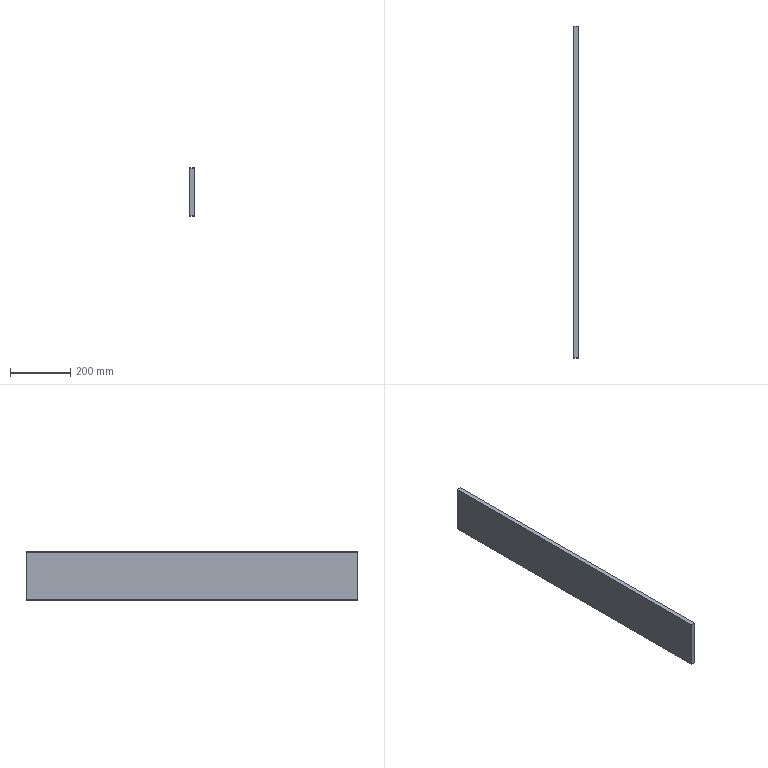Part | STEP file | HJDX-204 | 1 solid | 26 faces | box 16 x 1100 x 160 mm | volume 2815363 mm3 | plane 26
STEP:
#1=CARTESIAN_POINT('',(16.,-549.5,-79.5));
#2=VERTEX_POINT('',#1);
#3=CARTESIAN_POINT('',(16.,-549.5,79.5));
#4=VERTEX_POINT('',#3);
#5=CARTESIAN_POINT('',(16.,-549.5,0.));
#6=DIRECTION('',(0.,0.,1.));
#7=VECTOR('',#6,1000.);
#8=LINE('',#5,#7);
#9=EDGE_CURVE('',#2,#4,#8,.T.);
#10=ORIENTED_EDGE('',*,*,#9,.F.);
#11=CARTESIAN_POINT('',(16.,549.5,-79.5));
#12=VERTEX_POINT('',#11);
#13=CARTESIAN_POINT('',(16.,0.,-79.5));
#14=DIRECTION('',(0.,-1.,0.));
#15=VECTOR('',#14,1000.);
#16=LINE('',#13,#15);
#17=EDGE_CURVE('',#12,#2,#16,.T.);
#18=ORIENTED_EDGE('',*,*,#17,.F.);
#19=CARTESIAN_POINT('',(16.,549.5,79.5));
#20=VERTEX_POINT('',#19);
#21=CARTESIAN_POINT('',(16.,549.5,0.));
#22=DIRECTION('',(0.,0.,-1.));
#23=VECTOR('',#22,1000.);
#24=LINE('',#21,#23);
#25=EDGE_CURVE('',#20,#12,#24,.T.);
#26=ORIENTED_EDGE('',*,*,#25,.F.);
#27=CARTESIAN_POINT('',(16.,0.,79.5));
#28=DIRECTION('',(0.,1.,0.));
#29=VECTOR('',#28,1000.);
#30=LINE('',#27,#29);
#31=EDGE_CURVE('',#4,#20,#30,.T.);
#32=ORIENTED_EDGE('',*,*,#31,.F.);
#33=EDGE_LOOP('',(#10,#18,#26,#32));
#34=FACE_OUTER_BOUND('',#33,.T.);
#35=CARTESIAN_POINT('',(16.,0.,0.));
#36=DIRECTION('',(-1.,0.,0.));
#37=DIRECTION('',(0.,0.,1.));
#38=AXIS2_PLACEMENT_3D('',#35,#36,#37);
#39=PLANE('',#38);
#40=ADVANCED_FACE('',(#34),#39,.F.);
#41=CARTESIAN_POINT('',(15.5,-549.5,80.));
#42=VERTEX_POINT('',#41);
#43=CARTESIAN_POINT('',(15.5,549.5,80.));
#44=VERTEX_POINT('',#43);
#45=CARTESIAN_POINT('',(15.5,0.,80.));
#46=DIRECTION('',(0.,1.,0.));
#47=VECTOR('',#46,1000.);
#48=LINE('',#45,#47);
#49=EDGE_CURVE('',#42,#44,#48,.T.);
#50=ORIENTED_EDGE('',*,*,#49,.F.);
#51=CARTESIAN_POINT('',(16.,-549.5,79.5));
#52=DIRECTION('',(-0.7071,0.,0.7071));
#53=VECTOR('',#52,1000.);
#54=LINE('',#51,#53);
#55=EDGE_CURVE('',#4,#42,#54,.T.);
#56=ORIENTED_EDGE('',*,*,#55,.F.);
#57=ORIENTED_EDGE('',*,*,#31,.T.);
#58=CARTESIAN_POINT('',(16.,549.5,79.5));
#59=DIRECTION('',(0.7071,0.,-0.7071));
#60=VECTOR('',#59,1000.);
#61=LINE('',#58,#60);
#62=EDGE_CURVE('',#44,#20,#61,.T.);
#63=ORIENTED_EDGE('',*,*,#62,.F.);
#64=EDGE_LOOP('',(#50,#56,#57,#63));
#65=FACE_OUTER_BOUND('',#64,.T.);
#66=CARTESIAN_POINT('',(16.,0.,79.5));
#67=DIRECTION('',(-0.7071,0.,-0.7071));
#68=DIRECTION('',(-0.7071,0.,0.7071));
#69=AXIS2_PLACEMENT_3D('',#66,#67,#68);
#70=PLANE('',#69);
#71=ADVANCED_FACE('',(#65),#70,.F.);
#72=CARTESIAN_POINT('',(15.5,-550.,-79.5));
#73=VERTEX_POINT('',#72);
#74=CARTESIAN_POINT('',(15.5,-550.,79.5));
#75=VERTEX_POINT('',#74);
#76=CARTESIAN_POINT('',(15.5,-550.,0.));
#77=DIRECTION('',(0.,0.,1.));
#78=VECTOR('',#77,1000.);
#79=LINE('',#76,#78);
#80=EDGE_CURVE('',#73,#75,#79,.T.);
#81=ORIENTED_EDGE('',*,*,#80,.F.);
#82=CARTESIAN_POINT('',(16.,-549.5,-79.5));
#83=DIRECTION('',(-0.7071,-0.7071,0.));
#84=VECTOR('',#83,1000.);
#85=LINE('',#82,#84);
#86=EDGE_CURVE('',#2,#73,#85,.T.);
#87=ORIENTED_EDGE('',*,*,#86,.F.);
#88=ORIENTED_EDGE('',*,*,#9,.T.);
#89=CARTESIAN_POINT('',(16.,-549.5,79.5));
#90=DIRECTION('',(0.7071,0.7071,0.));
#91=VECTOR('',#90,1000.);
#92=LINE('',#89,#91);
#93=EDGE_CURVE('',#75,#4,#92,.T.);
#94=ORIENTED_EDGE('',*,*,#93,.F.);
#95=EDGE_LOOP('',(#81,#87,#88,#94));
#96=FACE_OUTER_BOUND('',#95,.T.);
#97=CARTESIAN_POINT('',(16.,-549.5,0.));
#98=DIRECTION('',(-0.7071,0.7071,0.));
#99=DIRECTION('',(-0.7071,-0.7071,0.));
#100=AXIS2_PLACEMENT_3D('',#97,#98,#99);
#101=PLANE('',#100);
#102=ADVANCED_FACE('',(#96),#101,.F.);
#103=ORIENTED_EDGE('',*,*,#17,.T.);
#104=CARTESIAN_POINT('',(15.5,-549.5,-80.));
#105=VERTEX_POINT('',#104);
#106=CARTESIAN_POINT('',(16.,-549.5,-79.5));
#107=DIRECTION('',(0.7071,0.,0.7071));
#108=VECTOR('',#107,1000.);
#109=LINE('',#106,#108);
#110=EDGE_CURVE('',#105,#2,#109,.T.);
#111=ORIENTED_EDGE('',*,*,#110,.F.);
#112=CARTESIAN_POINT('',(15.5,549.5,-80.));
#113=VERTEX_POINT('',#112);
#114=CARTESIAN_POINT('',(15.5,0.,-80.));
#115=DIRECTION('',(0.,-1.,0.));
#116=VECTOR('',#115,1000.);
#117=LINE('',#114,#116);
#118=EDGE_CURVE('',#113,#105,#117,.T.);
#119=ORIENTED_EDGE('',*,*,#118,.F.);
#120=CARTESIAN_POINT('',(16.,549.5,-79.5));
#121=DIRECTION('',(-0.7071,0.,-0.7071));
#122=VECTOR('',#121,1000.);
#123=LINE('',#120,#122);
#124=EDGE_CURVE('',#12,#113,#123,.T.);
#125=ORIENTED_EDGE('',*,*,#124,.F.);
#126=EDGE_LOOP('',(#103,#111,#119,#125));
#127=FACE_OUTER_BOUND('',#126,.T.);
#128=CARTESIAN_POINT('',(16.,0.,-79.5));
#129=DIRECTION('',(-0.7071,0.,0.7071));
#130=DIRECTION('',(0.7071,0.,0.7071));
#131=AXIS2_PLACEMENT_3D('',#128,#129,#130);
#132=PLANE('',#131);
#133=ADVANCED_FACE('',(#127),#132,.F.);
#134=ORIENTED_EDGE('',*,*,#25,.T.);
#135=CARTESIAN_POINT('',(15.5,550.,-79.5));
#136=VERTEX_POINT('',#135);
#137=CARTESIAN_POINT('',(16.,549.5,-79.5));
#138=DIRECTION('',(0.7071,-0.7071,0.));
#139=VECTOR('',#138,1000.);
#140=LINE('',#137,#139);
#141=EDGE_CURVE('',#136,#12,#140,.T.);
#142=ORIENTED_EDGE('',*,*,#141,.F.);
#143=CARTESIAN_POINT('',(15.5,550.,79.5));
#144=VERTEX_POINT('',#143);
#145=CARTESIAN_POINT('',(15.5,550.,0.));
#146=DIRECTION('',(0.,0.,-1.));
#147=VECTOR('',#146,1000.);
#148=LINE('',#145,#147);
#149=EDGE_CURVE('',#144,#136,#148,.T.);
#150=ORIENTED_EDGE('',*,*,#149,.F.);
#151=CARTESIAN_POINT('',(16.,549.5,79.5));
#152=DIRECTION('',(-0.7071,0.7071,0.));
#153=VECTOR('',#152,1000.);
#154=LINE('',#151,#153);
#155=EDGE_CURVE('',#20,#144,#154,.T.);
#156=ORIENTED_EDGE('',*,*,#155,.F.);
#157=EDGE_LOOP('',(#134,#142,#150,#156));
#158=FACE_OUTER_BOUND('',#157,.T.);
#159=CARTESIAN_POINT('',(16.,549.5,0.));
#160=DIRECTION('',(-0.7071,-0.7071,0.));
#161=DIRECTION('',(0.7071,-0.7071,0.));
#162=AXIS2_PLACEMENT_3D('',#159,#160,#161);
#163=PLANE('',#162);
#164=ADVANCED_FACE('',(#158),#163,.F.);
#165=CARTESIAN_POINT('',(15.5,549.5,80.));
#166=DIRECTION('',(0.,-0.7071,0.7071));
#167=VECTOR('',#166,1000.);
#168=LINE('',#165,#167);
#169=EDGE_CURVE('',#144,#44,#168,.T.);
#170=ORIENTED_EDGE('',*,*,#169,.T.);
#171=ORIENTED_EDGE('',*,*,#62,.T.);
#172=ORIENTED_EDGE('',*,*,#155,.T.);
#173=EDGE_LOOP('',(#170,#171,#172));
#174=FACE_OUTER_BOUND('',#173,.T.);
#175=CARTESIAN_POINT('',(15.5,550.,79.5));
#176=DIRECTION('',(0.5774,0.5774,0.5774));
#177=DIRECTION('',(0.7071,0.,-0.7071));
#178=AXIS2_PLACEMENT_3D('',#175,#176,#177);
#179=PLANE('',#178);
#180=ADVANCED_FACE('',(#174),#179,.T.);
#181=CARTESIAN_POINT('',(0.5,549.5,80.));
#182=VERTEX_POINT('',#181);
#183=CARTESIAN_POINT('',(16.,549.5,80.));
#184=DIRECTION('',(1.,0.,0.));
#185=VECTOR('',#184,1000.);
#186=LINE('',#183,#185);
#187=EDGE_CURVE('',#182,#44,#186,.T.);
#188=ORIENTED_EDGE('',*,*,#187,.F.);
#189=CARTESIAN_POINT('',(0.5,-549.5,80.));
#190=VERTEX_POINT('',#189);
#191=CARTESIAN_POINT('',(0.5,-550.,80.));
#192=DIRECTION('',(0.,1.,0.));
#193=VECTOR('',#192,1000.);
#194=LINE('',#191,#193);
#195=EDGE_CURVE('',#190,#182,#194,.T.);
#196=ORIENTED_EDGE('',*,*,#195,.F.);
#197=CARTESIAN_POINT('',(16.,-549.5,80.));
#198=DIRECTION('',(-1.,0.,0.));
#199=VECTOR('',#198,1000.);
#200=LINE('',#197,#199);
#201=EDGE_CURVE('',#42,#190,#200,.T.);
#202=ORIENTED_EDGE('',*,*,#201,.F.);
#203=ORIENTED_EDGE('',*,*,#49,.T.);
#204=EDGE_LOOP('',(#188,#196,#202,#203));
#205=FACE_OUTER_BOUND('',#204,.T.);
#206=CARTESIAN_POINT('',(16.,-550.,80.));
#207=DIRECTION('',(0.,0.,-1.));
#208=DIRECTION('',(-1.,0.,0.));
#209=AXIS2_PLACEMENT_3D('',#206,#207,#208);
#210=PLANE('',#209);
#211=ADVANCED_FACE('',(#205),#210,.F.);
#212=CARTESIAN_POINT('',(15.5,-549.5,80.));
#213=DIRECTION('',(0.,-0.7071,-0.7071));
#214=VECTOR('',#213,1000.);
#215=LINE('',#212,#214);
#216=EDGE_CURVE('',#42,#75,#215,.T.);
#217=ORIENTED_EDGE('',*,*,#216,.T.);
#218=ORIENTED_EDGE('',*,*,#93,.T.);
#219=ORIENTED_EDGE('',*,*,#55,.T.);
#220=EDGE_LOOP('',(#217,#218,#219));
#221=FACE_OUTER_BOUND('',#220,.T.);
#222=CARTESIAN_POINT('',(15.5,-549.5,80.));
#223=DIRECTION('',(0.5774,-0.5774,0.5774));
#224=DIRECTION('',(0.7071,0.,-0.7071));
#225=AXIS2_PLACEMENT_3D('',#222,#223,#224);
#226=PLANE('',#225);
#227=ADVANCED_FACE('',(#221),#226,.T.);
#228=CARTESIAN_POINT('',(0.5,-550.,-79.5));
#229=VERTEX_POINT('',#228);
#230=CARTESIAN_POINT('',(16.,-550.,-79.5));
#231=DIRECTION('',(-1.,0.,0.));
#232=VECTOR('',#231,1000.);
#233=LINE('',#230,#232);
#234=EDGE_CURVE('',#73,#229,#233,.T.);
#235=ORIENTED_EDGE('',*,*,#234,.F.);
#236=ORIENTED_EDGE('',*,*,#80,.T.);
#237=CARTESIAN_POINT('',(0.5,-550.,79.5));
#238=VERTEX_POINT('',#237);
#239=CARTESIAN_POINT('',(16.,-550.,79.5));
#240=DIRECTION('',(1.,0.,0.));
#241=VECTOR('',#240,1000.);
#242=LINE('',#239,#241);
#243=EDGE_CURVE('',#238,#75,#242,.T.);
#244=ORIENTED_EDGE('',*,*,#243,.F.);
#245=CARTESIAN_POINT('',(0.5,-550.,80.));
#246=DIRECTION('',(0.,0.,1.));
#247=VECTOR('',#246,1000.);
#248=LINE('',#245,#247);
#249=EDGE_CURVE('',#229,#238,#248,.T.);
#250=ORIENTED_EDGE('',*,*,#249,.F.);
#251=EDGE_LOOP('',(#235,#236,#244,#250));
#252=FACE_OUTER_BOUND('',#251,.T.);
#253=CARTESIAN_POINT('',(16.,-550.,80.));
#254=DIRECTION('',(0.,1.,0.));
#255=DIRECTION('',(0.,0.,1.));
#256=AXIS2_PLACEMENT_3D('',#253,#254,#255);
#257=PLANE('',#256);
#258=ADVANCED_FACE('',(#252),#257,.F.);
#259=ORIENTED_EDGE('',*,*,#86,.T.);
#260=CARTESIAN_POINT('',(15.5,-550.,-79.5));
#261=DIRECTION('',(0.,0.7071,-0.7071));
#262=VECTOR('',#261,1000.);
#263=LINE('',#260,#262);
#264=EDGE_CURVE('',#73,#105,#263,.T.);
#265=ORIENTED_EDGE('',*,*,#264,.T.);
#266=ORIENTED_EDGE('',*,*,#110,.T.);
#267=EDGE_LOOP('',(#259,#265,#266));
#268=FACE_OUTER_BOUND('',#267,.T.);
#269=CARTESIAN_POINT('',(15.5,-550.,-79.5));
#270=DIRECTION('',(0.5774,-0.5774,-0.5774));
#271=DIRECTION('',(-0.7071,0.,-0.7071));
#272=AXIS2_PLACEMENT_3D('',#269,#270,#271);
#273=PLANE('',#272);
#274=ADVANCED_FACE('',(#268),#273,.T.);
#275=ORIENTED_EDGE('',*,*,#141,.T.);
#276=ORIENTED_EDGE('',*,*,#124,.T.);
#277=CARTESIAN_POINT('',(15.5,550.,-79.5));
#278=DIRECTION('',(0.,0.7071,0.7071));
#279=VECTOR('',#278,1000.);
#280=LINE('',#277,#279);
#281=EDGE_CURVE('',#113,#136,#280,.T.);
#282=ORIENTED_EDGE('',*,*,#281,.T.);
#283=EDGE_LOOP('',(#275,#276,#282));
#284=FACE_OUTER_BOUND('',#283,.T.);
#285=CARTESIAN_POINT('',(15.5,549.5,-80.));
#286=DIRECTION('',(0.5774,0.5774,-0.5774));
#287=DIRECTION('',(-0.7071,0.,-0.7071));
#288=AXIS2_PLACEMENT_3D('',#285,#286,#287);
#289=PLANE('',#288);
#290=ADVANCED_FACE('',(#284),#289,.T.);
#291=CARTESIAN_POINT('',(0.5,549.5,-80.));
#292=VERTEX_POINT('',#291);
#293=CARTESIAN_POINT('',(0.5,-549.5,-80.));
#294=VERTEX_POINT('',#293);
#295=CARTESIAN_POINT('',(0.5,-550.,-80.));
#296=DIRECTION('',(0.,-1.,0.));
#297=VECTOR('',#296,1000.);
#298=LINE('',#295,#297);
#299=EDGE_CURVE('',#292,#294,#298,.T.);
#300=ORIENTED_EDGE('',*,*,#299,.F.);
#301=CARTESIAN_POINT('',(16.,549.5,-80.));
#302=DIRECTION('',(-1.,0.,0.));
#303=VECTOR('',#302,1000.);
#304=LINE('',#301,#303);
#305=EDGE_CURVE('',#113,#292,#304,.T.);
#306=ORIENTED_EDGE('',*,*,#305,.F.);
#307=ORIENTED_EDGE('',*,*,#118,.T.);
#308=CARTESIAN_POINT('',(16.,-549.5,-80.));
#309=DIRECTION('',(1.,0.,0.));
#310=VECTOR('',#309,1000.);
#311=LINE('',#308,#310);
#312=EDGE_CURVE('',#294,#105,#311,.T.);
#313=ORIENTED_EDGE('',*,*,#312,.F.);
#314=EDGE_LOOP('',(#300,#306,#307,#313));
#315=FACE_OUTER_BOUND('',#314,.T.);
#316=CARTESIAN_POINT('',(16.,-550.,-80.));
#317=DIRECTION('',(0.,0.,1.));
#318=DIRECTION('',(1.,0.,0.));
#319=AXIS2_PLACEMENT_3D('',#316,#317,#318);
#320=PLANE('',#319);
#321=ADVANCED_FACE('',(#315),#320,.F.);
#322=CARTESIAN_POINT('',(0.5,550.,79.5));
#323=VERTEX_POINT('',#322);
#324=CARTESIAN_POINT('',(0.5,550.,-79.5));
#325=VERTEX_POINT('',#324);
#326=CARTESIAN_POINT('',(0.5,550.,80.));
#327=DIRECTION('',(0.,0.,-1.));
#328=VECTOR('',#327,1000.);
#329=LINE('',#326,#328);
#330=EDGE_CURVE('',#323,#325,#329,.T.);
#331=ORIENTED_EDGE('',*,*,#330,.F.);
#332=CARTESIAN_POINT('',(16.,550.,79.5));
#333=DIRECTION('',(-1.,0.,0.));
#334=VECTOR('',#333,1000.);
#335=LINE('',#332,#334);
#336=EDGE_CURVE('',#144,#323,#335,.T.);
#337=ORIENTED_EDGE('',*,*,#336,.F.);
#338=ORIENTED_EDGE('',*,*,#149,.T.);
#339=CARTESIAN_POINT('',(16.,550.,-79.5));
#340=DIRECTION('',(1.,0.,0.));
#341=VECTOR('',#340,1000.);
#342=LINE('',#339,#341);
#343=EDGE_CURVE('',#325,#136,#342,.T.);
#344=ORIENTED_EDGE('',*,*,#343,.F.);
#345=EDGE_LOOP('',(#331,#337,#338,#344));
#346=FACE_OUTER_BOUND('',#345,.T.);
#347=CARTESIAN_POINT('',(16.,550.,80.));
#348=DIRECTION('',(0.,-1.,0.));
#349=DIRECTION('',(0.,0.,-1.));
#350=AXIS2_PLACEMENT_3D('',#347,#348,#349);
#351=PLANE('',#350);
#352=ADVANCED_FACE('',(#346),#351,.F.);
#353=ORIENTED_EDGE('',*,*,#336,.T.);
#354=CARTESIAN_POINT('',(0.5,549.5,80.));
#355=DIRECTION('',(0.,0.7071,-0.7071));
#356=VECTOR('',#355,1000.);
#357=LINE('',#354,#356);
#358=EDGE_CURVE('',#182,#323,#357,.T.);
#359=ORIENTED_EDGE('',*,*,#358,.F.);
#360=ORIENTED_EDGE('',*,*,#187,.T.);
#361=ORIENTED_EDGE('',*,*,#169,.F.);
#362=EDGE_LOOP('',(#353,#359,#360,#361));
#363=FACE_OUTER_BOUND('',#362,.T.);
#364=CARTESIAN_POINT('',(16.,549.5,80.));
#365=DIRECTION('',(0.,-0.7071,-0.7071));
#366=DIRECTION('',(0.,0.7071,-0.7071));
#367=AXIS2_PLACEMENT_3D('',#364,#365,#366);
#368=PLANE('',#367);
#369=ADVANCED_FACE('',(#363),#368,.F.);
#370=CARTESIAN_POINT('',(0.,-549.5,79.5));
#371=VERTEX_POINT('',#370);
#372=CARTESIAN_POINT('',(0.5,-549.5,80.));
#373=DIRECTION('',(0.7071,0.,0.7071));
#374=VECTOR('',#373,1000.);
#375=LINE('',#372,#374);
#376=EDGE_CURVE('',#371,#190,#375,.T.);
#377=ORIENTED_EDGE('',*,*,#376,.T.);
#378=ORIENTED_EDGE('',*,*,#195,.T.);
#379=CARTESIAN_POINT('',(0.,549.5,79.5));
#380=VERTEX_POINT('',#379);
#381=CARTESIAN_POINT('',(0.5,549.5,80.));
#382=DIRECTION('',(-0.7071,0.,-0.7071));
#383=VECTOR('',#382,1000.);
#384=LINE('',#381,#383);
#385=EDGE_CURVE('',#182,#380,#384,.T.);
#386=ORIENTED_EDGE('',*,*,#385,.T.);
#387=CARTESIAN_POINT('',(0.,-550.,79.5));
#388=DIRECTION('',(0.,-1.,0.));
#389=VECTOR('',#388,1000.);
#390=LINE('',#387,#389);
#391=EDGE_CURVE('',#380,#371,#390,.T.);
#392=ORIENTED_EDGE('',*,*,#391,.T.);
#393=EDGE_LOOP('',(#377,#378,#386,#392));
#394=FACE_OUTER_BOUND('',#393,.T.);
#395=CARTESIAN_POINT('',(0.5,-550.,80.));
#396=DIRECTION('',(-0.7071,0.,0.7071));
#397=DIRECTION('',(0.7071,0.,0.7071));
#398=AXIS2_PLACEMENT_3D('',#395,#396,#397);
#399=PLANE('',#398);
#400=ADVANCED_FACE('',(#394),#399,.T.);
#401=ORIENTED_EDGE('',*,*,#201,.T.);
#402=CARTESIAN_POINT('',(0.5,-550.,79.5));
#403=DIRECTION('',(0.,0.7071,0.7071));
#404=VECTOR('',#403,1000.);
#405=LINE('',#402,#404);
#406=EDGE_CURVE('',#238,#190,#405,.T.);
#407=ORIENTED_EDGE('',*,*,#406,.F.);
#408=ORIENTED_EDGE('',*,*,#243,.T.);
#409=ORIENTED_EDGE('',*,*,#216,.F.);
#410=EDGE_LOOP('',(#401,#407,#408,#409));
#411=FACE_OUTER_BOUND('',#410,.T.);
#412=CARTESIAN_POINT('',(16.,-550.,79.5));
#413=DIRECTION('',(0.,0.7071,-0.7071));
#414=DIRECTION('',(0.,0.7071,0.7071));
#415=AXIS2_PLACEMENT_3D('',#412,#413,#414);
#416=PLANE('',#415);
#417=ADVANCED_FACE('',(#411),#416,.F.);
#418=CARTESIAN_POINT('',(0.,-549.5,-79.5));
#419=VERTEX_POINT('',#418);
#420=CARTESIAN_POINT('',(0.5,-550.,-79.5));
#421=DIRECTION('',(0.7071,-0.7071,0.));
#422=VECTOR('',#421,1000.);
#423=LINE('',#420,#422);
#424=EDGE_CURVE('',#419,#229,#423,.T.);
#425=ORIENTED_EDGE('',*,*,#424,.T.);
#426=ORIENTED_EDGE('',*,*,#249,.T.);
#427=CARTESIAN_POINT('',(0.5,-550.,79.5));
#428=DIRECTION('',(-0.7071,0.7071,0.));
#429=VECTOR('',#428,1000.);
#430=LINE('',#427,#429);
#431=EDGE_CURVE('',#238,#371,#430,.T.);
#432=ORIENTED_EDGE('',*,*,#431,.T.);
#433=CARTESIAN_POINT('',(0.,-549.5,80.));
#434=DIRECTION('',(0.,0.,-1.));
#435=VECTOR('',#434,1000.);
#436=LINE('',#433,#435);
#437=EDGE_CURVE('',#371,#419,#436,.T.);
#438=ORIENTED_EDGE('',*,*,#437,.T.);
#439=EDGE_LOOP('',(#425,#426,#432,#438));
#440=FACE_OUTER_BOUND('',#439,.T.);
#441=CARTESIAN_POINT('',(0.5,-550.,80.));
#442=DIRECTION('',(-0.7071,-0.7071,0.));
#443=DIRECTION('',(0.7071,-0.7071,0.));
#444=AXIS2_PLACEMENT_3D('',#441,#442,#443);
#445=PLANE('',#444);
#446=ADVANCED_FACE('',(#440),#445,.T.);
#447=ORIENTED_EDGE('',*,*,#234,.T.);
#448=CARTESIAN_POINT('',(0.5,-549.5,-80.));
#449=DIRECTION('',(0.,-0.7071,0.7071));
#450=VECTOR('',#449,1000.);
#451=LINE('',#448,#450);
#452=EDGE_CURVE('',#294,#229,#451,.T.);
#453=ORIENTED_EDGE('',*,*,#452,.F.);
#454=ORIENTED_EDGE('',*,*,#312,.T.);
#455=ORIENTED_EDGE('',*,*,#264,.F.);
#456=EDGE_LOOP('',(#447,#453,#454,#455));
#457=FACE_OUTER_BOUND('',#456,.T.);
#458=CARTESIAN_POINT('',(16.,-549.5,-80.));
#459=DIRECTION('',(0.,0.7071,0.7071));
#460=DIRECTION('',(0.,-0.7071,0.7071));
#461=AXIS2_PLACEMENT_3D('',#458,#459,#460);
#462=PLANE('',#461);
#463=ADVANCED_FACE('',(#457),#462,.F.);
#464=CARTESIAN_POINT('',(0.5,-549.5,-80.));
#465=DIRECTION('',(-0.7071,0.,0.7071));
#466=VECTOR('',#465,1000.);
#467=LINE('',#464,#466);
#468=EDGE_CURVE('',#294,#419,#467,.T.);
#469=ORIENTED_EDGE('',*,*,#468,.T.);
#470=CARTESIAN_POINT('',(0.,549.5,-79.5));
#471=VERTEX_POINT('',#470);
#472=CARTESIAN_POINT('',(0.,-550.,-79.5));
#473=DIRECTION('',(0.,1.,0.));
#474=VECTOR('',#473,1000.);
#475=LINE('',#472,#474);
#476=EDGE_CURVE('',#419,#471,#475,.T.);
#477=ORIENTED_EDGE('',*,*,#476,.T.);
#478=CARTESIAN_POINT('',(0.5,549.5,-80.));
#479=DIRECTION('',(0.7071,0.,-0.7071));
#480=VECTOR('',#479,1000.);
#481=LINE('',#478,#480);
#482=EDGE_CURVE('',#471,#292,#481,.T.);
#483=ORIENTED_EDGE('',*,*,#482,.T.);
#484=ORIENTED_EDGE('',*,*,#299,.T.);
#485=EDGE_LOOP('',(#469,#477,#483,#484));
#486=FACE_OUTER_BOUND('',#485,.T.);
#487=CARTESIAN_POINT('',(0.5,-550.,-80.));
#488=DIRECTION('',(-0.7071,0.,-0.7071));
#489=DIRECTION('',(-0.7071,0.,0.7071));
#490=AXIS2_PLACEMENT_3D('',#487,#488,#489);
#491=PLANE('',#490);
#492=ADVANCED_FACE('',(#486),#491,.T.);
#493=ORIENTED_EDGE('',*,*,#343,.T.);
#494=ORIENTED_EDGE('',*,*,#281,.F.);
#495=ORIENTED_EDGE('',*,*,#305,.T.);
#496=CARTESIAN_POINT('',(0.5,550.,-79.5));
#497=DIRECTION('',(0.,-0.7071,-0.7071));
#498=VECTOR('',#497,1000.);
#499=LINE('',#496,#498);
#500=EDGE_CURVE('',#325,#292,#499,.T.);
#501=ORIENTED_EDGE('',*,*,#500,.F.);
#502=EDGE_LOOP('',(#493,#494,#495,#501));
#503=FACE_OUTER_BOUND('',#502,.T.);
#504=CARTESIAN_POINT('',(16.,550.,-79.5));
#505=DIRECTION('',(0.,-0.7071,0.7071));
#506=DIRECTION('',(0.,-0.7071,-0.7071));
#507=AXIS2_PLACEMENT_3D('',#504,#505,#506);
#508=PLANE('',#507);
#509=ADVANCED_FACE('',(#503),#508,.F.);
#510=CARTESIAN_POINT('',(0.5,550.,-79.5));
#511=DIRECTION('',(-0.7071,-0.7071,0.));
#512=VECTOR('',#511,1000.);
#513=LINE('',#510,#512);
#514=EDGE_CURVE('',#325,#471,#513,.T.);
#515=ORIENTED_EDGE('',*,*,#514,.T.);
#516=CARTESIAN_POINT('',(0.,549.5,80.));
#517=DIRECTION('',(0.,0.,1.));
#518=VECTOR('',#517,1000.);
#519=LINE('',#516,#518);
#520=EDGE_CURVE('',#471,#380,#519,.T.);
#521=ORIENTED_EDGE('',*,*,#520,.T.);
#522=CARTESIAN_POINT('',(0.5,550.,79.5));
#523=DIRECTION('',(0.7071,0.7071,0.));
#524=VECTOR('',#523,1000.);
#525=LINE('',#522,#524);
#526=EDGE_CURVE('',#380,#323,#525,.T.);
#527=ORIENTED_EDGE('',*,*,#526,.T.);
#528=ORIENTED_EDGE('',*,*,#330,.T.);
#529=EDGE_LOOP('',(#515,#521,#527,#528));
#530=FACE_OUTER_BOUND('',#529,.T.);
#531=CARTESIAN_POINT('',(0.5,550.,80.));
#532=DIRECTION('',(-0.7071,0.7071,0.));
#533=DIRECTION('',(-0.7071,-0.7071,0.));
#534=AXIS2_PLACEMENT_3D('',#531,#532,#533);
#535=PLANE('',#534);
#536=ADVANCED_FACE('',(#530),#535,.T.);
#537=ORIENTED_EDGE('',*,*,#358,.T.);
#538=ORIENTED_EDGE('',*,*,#526,.F.);
#539=ORIENTED_EDGE('',*,*,#385,.F.);
#540=EDGE_LOOP('',(#537,#538,#539));
#541=FACE_OUTER_BOUND('',#540,.T.);
#542=CARTESIAN_POINT('',(0.5,549.5,80.));
#543=DIRECTION('',(-0.5774,0.5774,0.5774));
#544=DIRECTION('',(0.7071,0.,0.7071));
#545=AXIS2_PLACEMENT_3D('',#542,#543,#544);
#546=PLANE('',#545);
#547=ADVANCED_FACE('',(#541),#546,.T.);
#548=ORIENTED_EDGE('',*,*,#376,.F.);
#549=ORIENTED_EDGE('',*,*,#431,.F.);
#550=ORIENTED_EDGE('',*,*,#406,.T.);
#551=EDGE_LOOP('',(#548,#549,#550));
#552=FACE_OUTER_BOUND('',#551,.T.);
#553=CARTESIAN_POINT('',(0.5,-549.5,80.));
#554=DIRECTION('',(-0.5774,-0.5774,0.5774));
#555=DIRECTION('',(0.7071,0.,0.7071));
#556=AXIS2_PLACEMENT_3D('',#553,#554,#555);
#557=PLANE('',#556);
#558=ADVANCED_FACE('',(#552),#557,.T.);
#559=ORIENTED_EDGE('',*,*,#476,.F.);
#560=ORIENTED_EDGE('',*,*,#437,.F.);
#561=ORIENTED_EDGE('',*,*,#391,.F.);
#562=ORIENTED_EDGE('',*,*,#520,.F.);
#563=EDGE_LOOP('',(#559,#560,#561,#562));
#564=FACE_OUTER_BOUND('',#563,.T.);
#565=CARTESIAN_POINT('',(0.,0.,0.));
#566=DIRECTION('',(-1.,0.,0.));
#567=DIRECTION('',(0.,0.,1.));
#568=AXIS2_PLACEMENT_3D('',#565,#566,#567);
#569=PLANE('',#568);
#570=ADVANCED_FACE('',(#564),#569,.T.);
#571=ORIENTED_EDGE('',*,*,#468,.F.);
#572=ORIENTED_EDGE('',*,*,#452,.T.);
#573=ORIENTED_EDGE('',*,*,#424,.F.);
#574=EDGE_LOOP('',(#571,#572,#573));
#575=FACE_OUTER_BOUND('',#574,.T.);
#576=CARTESIAN_POINT('',(0.5,-549.5,-80.));
#577=DIRECTION('',(-0.5774,-0.5774,-0.5774));
#578=DIRECTION('',(-0.7071,0.,0.7071));
#579=AXIS2_PLACEMENT_3D('',#576,#577,#578);
#580=PLANE('',#579);
#581=ADVANCED_FACE('',(#575),#580,.T.);
#582=ORIENTED_EDGE('',*,*,#500,.T.);
#583=ORIENTED_EDGE('',*,*,#482,.F.);
#584=ORIENTED_EDGE('',*,*,#514,.F.);
#585=EDGE_LOOP('',(#582,#583,#584));
#586=FACE_OUTER_BOUND('',#585,.T.);
#587=CARTESIAN_POINT('',(0.5,550.,-79.5));
#588=DIRECTION('',(-0.5774,0.5774,-0.5774));
#589=DIRECTION('',(-0.7071,0.,0.7071));
#590=AXIS2_PLACEMENT_3D('',#587,#588,#589);
#591=PLANE('',#590);
#592=ADVANCED_FACE('',(#586),#591,.T.);
#593=CLOSED_SHELL('',(#40,#71,#102,#133,#164,#180,#211,#227,#258,#274,#290,#321,#352,#369,#400,#417,#446,#463,#492,#509,#536,#547,#558,#570,#581,#592));
#594=MANIFOLD_SOLID_BREP('',#593);
#595=CARTESIAN_POINT('',(0.,0.,0.));
#596=DIRECTION('',(0.,0.,1.));
#597=DIRECTION('',(1.,0.,0.));
#598=AXIS2_PLACEMENT_3D('',#595,#596,#597);
#599=(LENGTH_UNIT()NAMED_UNIT(*)SI_UNIT(.MILLI.,.METRE.));
#600=UNCERTAINTY_MEASURE_WITH_UNIT(LENGTH_MEASURE(0.00001),#599,'','');
#601=(NAMED_UNIT(*)PLANE_ANGLE_UNIT()SI_UNIT($,.RADIAN.));
#602=(NAMED_UNIT(*)SI_UNIT($,.STERADIAN.)SOLID_ANGLE_UNIT());
#603=(GEOMETRIC_REPRESENTATION_CONTEXT(3)GLOBAL_UNCERTAINTY_ASSIGNED_CONTEXT((#600))GLOBAL_UNIT_ASSIGNED_CONTEXT((#599,#601,#602))REPRESENTATION_CONTEXT('',''));
#604=ADVANCED_BREP_SHAPE_REPRESENTATION('',(#594,#598),#603);